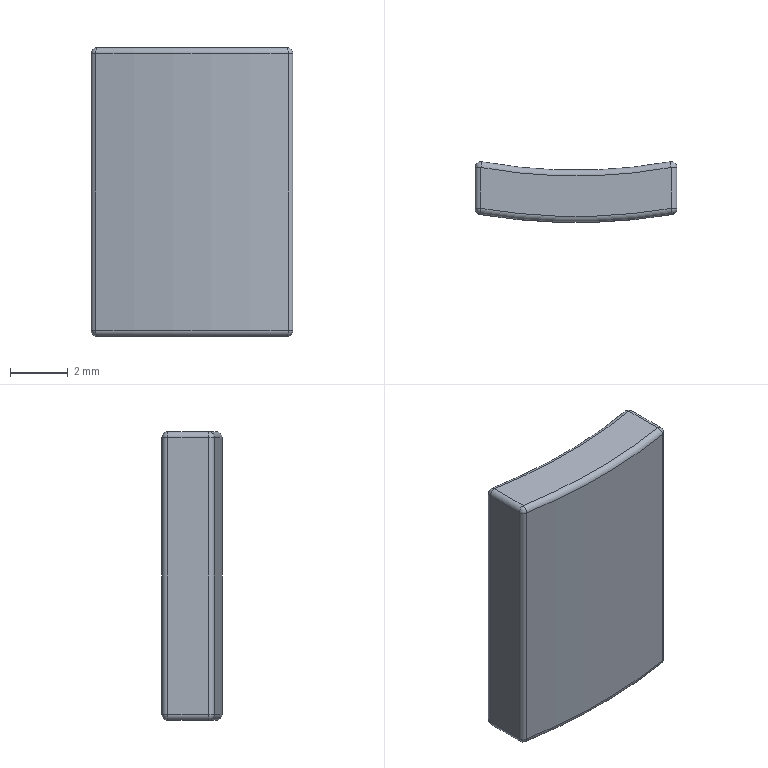Part | SolidWorks | features BaseBody 1 | 1 solid | 26 faces | box 7 x 2.098 x 10 mm | volume 126.049 mm3 | cylinder 10 | sphere 8 | plane 4 | torus 4 | commonest cylinder face diameters 0.4 x8 36.4 x1 40 x1
STEP:
#1=CARTESIAN_POINT('',(-3.3,-18.102,0.));
#2=VERTEX_POINT('',#1);
#3=CARTESIAN_POINT('',(3.3,-18.102,0.));
#4=VERTEX_POINT('',#3);
#5=CARTESIAN_POINT('',(0.,0.,0.));
#6=DIRECTION('',(0.,0.,1.));
#7=DIRECTION('',(-0.1793,-0.9838,0.));
#8=AXIS2_PLACEMENT_3D('',#5,#6,#7);
#9=CIRCLE('',#8,18.4);
#10=EDGE_CURVE('',#2,#4,#9,.T.);
#11=ORIENTED_EDGE('',*,*,#10,.F.);
#12=CARTESIAN_POINT('',(-3.3,-19.523,0.));
#13=VERTEX_POINT('',#12);
#14=CARTESIAN_POINT('',(-3.3,-19.523,0.));
#15=DIRECTION('',(0.,1.,0.));
#16=VECTOR('',#15,1000.);
#17=LINE('',#14,#16);
#18=EDGE_CURVE('',#13,#2,#17,.T.);
#19=ORIENTED_EDGE('',*,*,#18,.F.);
#20=CARTESIAN_POINT('',(3.3,-19.523,0.));
#21=VERTEX_POINT('',#20);
#22=CARTESIAN_POINT('',(0.,0.,0.));
#23=DIRECTION('',(0.,0.,-1.));
#24=DIRECTION('',(0.1667,-0.986,0.));
#25=AXIS2_PLACEMENT_3D('',#22,#23,#24);
#26=CIRCLE('',#25,19.8);
#27=EDGE_CURVE('',#21,#13,#26,.T.);
#28=ORIENTED_EDGE('',*,*,#27,.F.);
#29=CARTESIAN_POINT('',(3.3,-18.102,0.));
#30=DIRECTION('',(0.,-1.,0.));
#31=VECTOR('',#30,1000.);
#32=LINE('',#29,#31);
#33=EDGE_CURVE('',#4,#21,#32,.T.);
#34=ORIENTED_EDGE('',*,*,#33,.F.);
#35=EDGE_LOOP('',(#11,#19,#28,#34));
#36=FACE_OUTER_BOUND('',#35,.T.);
#37=CARTESIAN_POINT('',(0.,0.,0.));
#38=DIRECTION('',(0.,0.,1.));
#39=DIRECTION('',(1.,0.,0.));
#40=AXIS2_PLACEMENT_3D('',#37,#38,#39);
#41=PLANE('',#40);
#42=ADVANCED_FACE('',(#36),#41,.T.);
#43=CARTESIAN_POINT('',(3.3,-18.102,-10.));
#44=VERTEX_POINT('',#43);
#45=CARTESIAN_POINT('',(3.5,-18.102,-9.8));
#46=VERTEX_POINT('',#45);
#47=CARTESIAN_POINT('',(3.3,-18.102,-9.8));
#48=DIRECTION('',(0.,-1.,0.));
#49=DIRECTION('',(0.,0.,-1.));
#50=AXIS2_PLACEMENT_3D('',#47,#48,#49);
#51=CIRCLE('',#50,0.2);
#52=EDGE_CURVE('',#44,#46,#51,.T.);
#53=ORIENTED_EDGE('',*,*,#52,.F.);
#54=CARTESIAN_POINT('',(3.264,-17.905,-9.8));
#55=VERTEX_POINT('',#54);
#56=CARTESIAN_POINT('',(3.3,-18.102,-9.8));
#57=DIRECTION('',(0.9838,0.1793,0.));
#58=DIRECTION('',(0.,0.,-1.));
#59=AXIS2_PLACEMENT_3D('',#56,#57,#58);
#60=CIRCLE('',#59,0.2);
#61=EDGE_CURVE('',#44,#55,#60,.T.);
#62=ORIENTED_EDGE('',*,*,#61,.T.);
#63=CARTESIAN_POINT('',(3.3,-18.102,-9.8));
#64=DIRECTION('',(0.,0.,-1.));
#65=DIRECTION('',(-0.1793,0.9838,0.));
#66=AXIS2_PLACEMENT_3D('',#63,#64,#65);
#67=CIRCLE('',#66,0.2);
#68=EDGE_CURVE('',#55,#46,#67,.T.);
#69=ORIENTED_EDGE('',*,*,#68,.T.);
#70=EDGE_LOOP('',(#53,#62,#69));
#71=FACE_OUTER_BOUND('',#70,.T.);
#72=CARTESIAN_POINT('',(3.3,-18.102,-9.8));
#73=DIRECTION('',(0.,0.,-1.));
#74=DIRECTION('',(0.6406,0.7679,0.));
#75=AXIS2_PLACEMENT_3D('',#72,#73,#74);
#76=SPHERICAL_SURFACE('',#75,0.2);
#77=ADVANCED_FACE('',(#71),#76,.T.);
#78=CARTESIAN_POINT('',(-3.3,-18.102,-10.));
#79=VERTEX_POINT('',#78);
#80=CARTESIAN_POINT('',(-3.264,-17.905,-9.8));
#81=VERTEX_POINT('',#80);
#82=CARTESIAN_POINT('',(-3.3,-18.102,-9.8));
#83=DIRECTION('',(0.9838,-0.1793,0.));
#84=DIRECTION('',(0.,0.,-1.));
#85=AXIS2_PLACEMENT_3D('',#82,#83,#84);
#86=CIRCLE('',#85,0.2);
#87=EDGE_CURVE('',#79,#81,#86,.T.);
#88=ORIENTED_EDGE('',*,*,#87,.T.);
#89=CARTESIAN_POINT('',(0.,0.,-9.8));
#90=DIRECTION('',(0.,0.,1.));
#91=DIRECTION('',(-0.1793,-0.9838,0.));
#92=AXIS2_PLACEMENT_3D('',#89,#90,#91);
#93=CIRCLE('',#92,18.2);
#94=EDGE_CURVE('',#81,#55,#93,.T.);
#95=ORIENTED_EDGE('',*,*,#94,.T.);
#96=ORIENTED_EDGE('',*,*,#61,.F.);
#97=CARTESIAN_POINT('',(0.,0.,-10.));
#98=DIRECTION('',(0.,0.,1.));
#99=DIRECTION('',(-0.1793,-0.9838,0.));
#100=AXIS2_PLACEMENT_3D('',#97,#98,#99);
#101=CIRCLE('',#100,18.4);
#102=EDGE_CURVE('',#79,#44,#101,.T.);
#103=ORIENTED_EDGE('',*,*,#102,.F.);
#104=EDGE_LOOP('',(#88,#95,#96,#103));
#105=FACE_OUTER_BOUND('',#104,.T.);
#106=CARTESIAN_POINT('',(0.,0.,-9.8));
#107=DIRECTION('',(0.,0.,1.));
#108=DIRECTION('',(-0.1841,-0.9829,0.));
#109=AXIS2_PLACEMENT_3D('',#106,#107,#108);
#110=TOROIDAL_SURFACE('',#109,18.4,0.2);
#111=ADVANCED_FACE('',(#105),#110,.T.);
#112=ORIENTED_EDGE('',*,*,#87,.F.);
#113=CARTESIAN_POINT('',(-3.5,-18.102,-9.8));
#114=VERTEX_POINT('',#113);
#115=CARTESIAN_POINT('',(-3.3,-18.102,-9.8));
#116=DIRECTION('',(0.,1.,0.));
#117=DIRECTION('',(0.,0.,-1.));
#118=AXIS2_PLACEMENT_3D('',#115,#116,#117);
#119=CIRCLE('',#118,0.2);
#120=EDGE_CURVE('',#79,#114,#119,.T.);
#121=ORIENTED_EDGE('',*,*,#120,.T.);
#122=CARTESIAN_POINT('',(-3.3,-18.102,-9.8));
#123=DIRECTION('',(0.,0.,-1.));
#124=DIRECTION('',(-1.,0.,0.));
#125=AXIS2_PLACEMENT_3D('',#122,#123,#124);
#126=CIRCLE('',#125,0.2);
#127=EDGE_CURVE('',#114,#81,#126,.T.);
#128=ORIENTED_EDGE('',*,*,#127,.T.);
#129=EDGE_LOOP('',(#112,#121,#128));
#130=FACE_OUTER_BOUND('',#129,.T.);
#131=CARTESIAN_POINT('',(-3.3,-18.102,-9.8));
#132=DIRECTION('',(0.,0.,-1.));
#133=DIRECTION('',(-0.6406,0.7679,0.));
#134=AXIS2_PLACEMENT_3D('',#131,#132,#133);
#135=SPHERICAL_SURFACE('',#134,0.2);
#136=ADVANCED_FACE('',(#130),#135,.T.);
#137=CARTESIAN_POINT('',(-3.3,-19.523,-10.));
#138=VERTEX_POINT('',#137);
#139=CARTESIAN_POINT('',(-3.5,-19.523,-9.8));
#140=VERTEX_POINT('',#139);
#141=CARTESIAN_POINT('',(-3.3,-19.523,-9.8));
#142=DIRECTION('',(0.,1.,0.));
#143=DIRECTION('',(0.,0.,-1.));
#144=AXIS2_PLACEMENT_3D('',#141,#142,#143);
#145=CIRCLE('',#144,0.2);
#146=EDGE_CURVE('',#138,#140,#145,.T.);
#147=ORIENTED_EDGE('',*,*,#146,.T.);
#148=CARTESIAN_POINT('',(-3.5,-19.523,-9.8));
#149=DIRECTION('',(0.,1.,0.));
#150=VECTOR('',#149,1000.);
#151=LINE('',#148,#150);
#152=EDGE_CURVE('',#140,#114,#151,.T.);
#153=ORIENTED_EDGE('',*,*,#152,.T.);
#154=ORIENTED_EDGE('',*,*,#120,.F.);
#155=CARTESIAN_POINT('',(-3.3,-19.523,-10.));
#156=DIRECTION('',(0.,1.,0.));
#157=VECTOR('',#156,1000.);
#158=LINE('',#155,#157);
#159=EDGE_CURVE('',#138,#79,#158,.T.);
#160=ORIENTED_EDGE('',*,*,#159,.F.);
#161=EDGE_LOOP('',(#147,#153,#154,#160));
#162=FACE_OUTER_BOUND('',#161,.T.);
#163=CARTESIAN_POINT('',(-3.3,-19.649,-9.8));
#164=DIRECTION('',(0.,1.,0.));
#165=DIRECTION('',(0.,0.,-1.));
#166=AXIS2_PLACEMENT_3D('',#163,#164,#165);
#167=CYLINDRICAL_SURFACE('',#166,0.2);
#168=ADVANCED_FACE('',(#162),#167,.T.);
#169=CARTESIAN_POINT('',(-3.5,-18.102,-0.2));
#170=VERTEX_POINT('',#169);
#171=CARTESIAN_POINT('',(-3.5,-18.102,-9.8));
#172=DIRECTION('',(0.,0.,1.));
#173=VECTOR('',#172,1000.);
#174=LINE('',#171,#173);
#175=EDGE_CURVE('',#114,#170,#174,.T.);
#176=ORIENTED_EDGE('',*,*,#175,.F.);
#177=ORIENTED_EDGE('',*,*,#152,.F.);
#178=CARTESIAN_POINT('',(-3.5,-19.523,-0.2));
#179=VERTEX_POINT('',#178);
#180=CARTESIAN_POINT('',(-3.5,-19.523,-0.2));
#181=DIRECTION('',(0.,0.,-1.));
#182=VECTOR('',#181,1000.);
#183=LINE('',#180,#182);
#184=EDGE_CURVE('',#179,#140,#183,.T.);
#185=ORIENTED_EDGE('',*,*,#184,.F.);
#186=CARTESIAN_POINT('',(-3.5,-19.523,-0.2));
#187=DIRECTION('',(0.,1.,0.));
#188=VECTOR('',#187,1000.);
#189=LINE('',#186,#188);
#190=EDGE_CURVE('',#179,#170,#189,.T.);
#191=ORIENTED_EDGE('',*,*,#190,.T.);
#192=EDGE_LOOP('',(#176,#177,#185,#191));
#193=FACE_OUTER_BOUND('',#192,.T.);
#194=CARTESIAN_POINT('',(-3.5,-15.854,-10.));
#195=DIRECTION('',(1.,0.,0.));
#196=DIRECTION('',(0.,1.,0.));
#197=AXIS2_PLACEMENT_3D('',#194,#195,#196);
#198=PLANE('',#197);
#199=ADVANCED_FACE('',(#193),#198,.F.);
#200=CARTESIAN_POINT('',(-3.3,-19.523,-0.2));
#201=DIRECTION('',(0.,1.,0.));
#202=DIRECTION('',(-1.,0.,0.));
#203=AXIS2_PLACEMENT_3D('',#200,#201,#202);
#204=CIRCLE('',#203,0.2);
#205=EDGE_CURVE('',#179,#13,#204,.T.);
#206=ORIENTED_EDGE('',*,*,#205,.T.);
#207=ORIENTED_EDGE('',*,*,#18,.T.);
#208=CARTESIAN_POINT('',(-3.3,-18.102,-0.2));
#209=DIRECTION('',(0.,1.,0.));
#210=DIRECTION('',(-1.,0.,0.));
#211=AXIS2_PLACEMENT_3D('',#208,#209,#210);
#212=CIRCLE('',#211,0.2);
#213=EDGE_CURVE('',#170,#2,#212,.T.);
#214=ORIENTED_EDGE('',*,*,#213,.F.);
#215=ORIENTED_EDGE('',*,*,#190,.F.);
#216=EDGE_LOOP('',(#206,#207,#214,#215));
#217=FACE_OUTER_BOUND('',#216,.T.);
#218=CARTESIAN_POINT('',(-3.3,-19.608,-0.2));
#219=DIRECTION('',(0.,1.,0.));
#220=DIRECTION('',(-1.,0.,0.));
#221=AXIS2_PLACEMENT_3D('',#218,#219,#220);
#222=CYLINDRICAL_SURFACE('',#221,0.2);
#223=ADVANCED_FACE('',(#217),#222,.T.);
#224=ORIENTED_EDGE('',*,*,#213,.T.);
#225=CARTESIAN_POINT('',(-3.264,-17.905,-0.2));
#226=VERTEX_POINT('',#225);
#227=CARTESIAN_POINT('',(-3.3,-18.102,-0.2));
#228=DIRECTION('',(0.9838,-0.1793,0.));
#229=DIRECTION('',(0.1793,0.9838,0.));
#230=AXIS2_PLACEMENT_3D('',#227,#228,#229);
#231=CIRCLE('',#230,0.2);
#232=EDGE_CURVE('',#226,#2,#231,.T.);
#233=ORIENTED_EDGE('',*,*,#232,.F.);
#234=CARTESIAN_POINT('',(-3.3,-18.102,-0.2));
#235=DIRECTION('',(0.,0.,-1.));
#236=DIRECTION('',(-1.,0.,0.));
#237=AXIS2_PLACEMENT_3D('',#234,#235,#236);
#238=CIRCLE('',#237,0.2);
#239=EDGE_CURVE('',#170,#226,#238,.T.);
#240=ORIENTED_EDGE('',*,*,#239,.F.);
#241=EDGE_LOOP('',(#224,#233,#240));
#242=FACE_OUTER_BOUND('',#241,.T.);
#243=CARTESIAN_POINT('',(-3.3,-18.102,-0.2));
#244=DIRECTION('',(0.,0.,-1.));
#245=DIRECTION('',(-0.6406,0.7679,0.));
#246=AXIS2_PLACEMENT_3D('',#243,#244,#245);
#247=SPHERICAL_SURFACE('',#246,0.2);
#248=ADVANCED_FACE('',(#242),#247,.T.);
#249=CARTESIAN_POINT('',(-3.264,-17.905,-9.8));
#250=DIRECTION('',(0.,0.,1.));
#251=VECTOR('',#250,1000.);
#252=LINE('',#249,#251);
#253=EDGE_CURVE('',#81,#226,#252,.T.);
#254=ORIENTED_EDGE('',*,*,#253,.F.);
#255=ORIENTED_EDGE('',*,*,#127,.F.);
#256=ORIENTED_EDGE('',*,*,#175,.T.);
#257=ORIENTED_EDGE('',*,*,#239,.T.);
#258=EDGE_LOOP('',(#254,#255,#256,#257));
#259=FACE_OUTER_BOUND('',#258,.T.);
#260=CARTESIAN_POINT('',(-3.3,-18.102,-23.036));
#261=DIRECTION('',(0.,0.,1.));
#262=DIRECTION('',(0.1793,0.9838,0.));
#263=AXIS2_PLACEMENT_3D('',#260,#261,#262);
#264=CYLINDRICAL_SURFACE('',#263,0.2);
#265=ADVANCED_FACE('',(#259),#264,.T.);
#266=CARTESIAN_POINT('',(3.264,-17.905,-0.2));
#267=VERTEX_POINT('',#266);
#268=CARTESIAN_POINT('',(3.264,-17.905,-0.2));
#269=DIRECTION('',(0.,0.,-1.));
#270=VECTOR('',#269,1000.);
#271=LINE('',#268,#270);
#272=EDGE_CURVE('',#267,#55,#271,.T.);
#273=ORIENTED_EDGE('',*,*,#272,.T.);
#274=ORIENTED_EDGE('',*,*,#94,.F.);
#275=ORIENTED_EDGE('',*,*,#253,.T.);
#276=CARTESIAN_POINT('',(0.,0.,-0.2));
#277=DIRECTION('',(0.,0.,1.));
#278=DIRECTION('',(-0.1793,-0.9838,0.));
#279=AXIS2_PLACEMENT_3D('',#276,#277,#278);
#280=CIRCLE('',#279,18.2);
#281=EDGE_CURVE('',#226,#267,#280,.T.);
#282=ORIENTED_EDGE('',*,*,#281,.T.);
#283=EDGE_LOOP('',(#273,#274,#275,#282));
#284=FACE_OUTER_BOUND('',#283,.T.);
#285=CARTESIAN_POINT('',(0.,0.,-10.5));
#286=DIRECTION('',(0.,0.,1.));
#287=DIRECTION('',(-1.,0.,0.));
#288=AXIS2_PLACEMENT_3D('',#285,#286,#287);
#289=CYLINDRICAL_SURFACE('',#288,18.2);
#290=ADVANCED_FACE('',(#284),#289,.F.);
#291=ORIENTED_EDGE('',*,*,#232,.T.);
#292=ORIENTED_EDGE('',*,*,#10,.T.);
#293=CARTESIAN_POINT('',(3.3,-18.102,-0.2));
#294=DIRECTION('',(0.9838,0.1793,0.));
#295=DIRECTION('',(-0.1793,0.9838,0.));
#296=AXIS2_PLACEMENT_3D('',#293,#294,#295);
#297=CIRCLE('',#296,0.2);
#298=EDGE_CURVE('',#267,#4,#297,.T.);
#299=ORIENTED_EDGE('',*,*,#298,.F.);
#300=ORIENTED_EDGE('',*,*,#281,.F.);
#301=EDGE_LOOP('',(#291,#292,#299,#300));
#302=FACE_OUTER_BOUND('',#301,.T.);
#303=CARTESIAN_POINT('',(0.,0.,-0.2));
#304=DIRECTION('',(0.,0.,1.));
#305=DIRECTION('',(-0.1844,-0.9829,0.));
#306=AXIS2_PLACEMENT_3D('',#303,#304,#305);
#307=TOROIDAL_SURFACE('',#306,18.4,0.2);
#308=ADVANCED_FACE('',(#302),#307,.T.);
#309=ORIENTED_EDGE('',*,*,#298,.T.);
#310=CARTESIAN_POINT('',(3.5,-18.102,-0.2));
#311=VERTEX_POINT('',#310);
#312=CARTESIAN_POINT('',(3.3,-18.102,-0.2));
#313=DIRECTION('',(0.,-1.,0.));
#314=DIRECTION('',(1.,0.,0.));
#315=AXIS2_PLACEMENT_3D('',#312,#313,#314);
#316=CIRCLE('',#315,0.2);
#317=EDGE_CURVE('',#311,#4,#316,.T.);
#318=ORIENTED_EDGE('',*,*,#317,.F.);
#319=CARTESIAN_POINT('',(3.3,-18.102,-0.2));
#320=DIRECTION('',(0.,0.,-1.));
#321=DIRECTION('',(-0.1793,0.9838,0.));
#322=AXIS2_PLACEMENT_3D('',#319,#320,#321);
#323=CIRCLE('',#322,0.2);
#324=EDGE_CURVE('',#267,#311,#323,.T.);
#325=ORIENTED_EDGE('',*,*,#324,.F.);
#326=EDGE_LOOP('',(#309,#318,#325));
#327=FACE_OUTER_BOUND('',#326,.T.);
#328=CARTESIAN_POINT('',(3.3,-18.102,-0.2));
#329=DIRECTION('',(0.,0.,-1.));
#330=DIRECTION('',(0.6406,0.7679,0.));
#331=AXIS2_PLACEMENT_3D('',#328,#329,#330);
#332=SPHERICAL_SURFACE('',#331,0.2);
#333=ADVANCED_FACE('',(#327),#332,.T.);
#334=CARTESIAN_POINT('',(3.5,-18.102,-0.2));
#335=DIRECTION('',(0.,0.,-1.));
#336=VECTOR('',#335,1000.);
#337=LINE('',#334,#336);
#338=EDGE_CURVE('',#311,#46,#337,.T.);
#339=ORIENTED_EDGE('',*,*,#338,.T.);
#340=ORIENTED_EDGE('',*,*,#68,.F.);
#341=ORIENTED_EDGE('',*,*,#272,.F.);
#342=ORIENTED_EDGE('',*,*,#324,.T.);
#343=EDGE_LOOP('',(#339,#340,#341,#342));
#344=FACE_OUTER_BOUND('',#343,.T.);
#345=CARTESIAN_POINT('',(3.3,-18.102,13.036));
#346=DIRECTION('',(0.,0.,-1.));
#347=DIRECTION('',(-0.1793,0.9838,0.));
#348=AXIS2_PLACEMENT_3D('',#345,#346,#347);
#349=CYLINDRICAL_SURFACE('',#348,0.2);
#350=ADVANCED_FACE('',(#344),#349,.T.);
#351=CARTESIAN_POINT('',(3.5,-19.523,-9.8));
#352=VERTEX_POINT('',#351);
#353=CARTESIAN_POINT('',(3.5,-19.523,-0.2));
#354=VERTEX_POINT('',#353);
#355=CARTESIAN_POINT('',(3.5,-19.523,-9.8));
#356=DIRECTION('',(0.,0.,1.));
#357=VECTOR('',#356,1000.);
#358=LINE('',#355,#357);
#359=EDGE_CURVE('',#352,#354,#358,.T.);
#360=ORIENTED_EDGE('',*,*,#359,.F.);
#361=CARTESIAN_POINT('',(3.5,-18.102,-9.8));
#362=DIRECTION('',(0.,-1.,0.));
#363=VECTOR('',#362,1000.);
#364=LINE('',#361,#363);
#365=EDGE_CURVE('',#46,#352,#364,.T.);
#366=ORIENTED_EDGE('',*,*,#365,.F.);
#367=ORIENTED_EDGE('',*,*,#338,.F.);
#368=CARTESIAN_POINT('',(3.5,-18.102,-0.2));
#369=DIRECTION('',(0.,-1.,0.));
#370=VECTOR('',#369,1000.);
#371=LINE('',#368,#370);
#372=EDGE_CURVE('',#311,#354,#371,.T.);
#373=ORIENTED_EDGE('',*,*,#372,.T.);
#374=EDGE_LOOP('',(#360,#366,#367,#373));
#375=FACE_OUTER_BOUND('',#374,.T.);
#376=CARTESIAN_POINT('',(3.5,-22.259,-10.));
#377=DIRECTION('',(-1.,0.,0.));
#378=DIRECTION('',(0.,0.,1.));
#379=AXIS2_PLACEMENT_3D('',#376,#377,#378);
#380=PLANE('',#379);
#381=ADVANCED_FACE('',(#375),#380,.F.);
#382=ORIENTED_EDGE('',*,*,#317,.T.);
#383=ORIENTED_EDGE('',*,*,#33,.T.);
#384=CARTESIAN_POINT('',(3.3,-19.523,-0.2));
#385=DIRECTION('',(0.,-1.,0.));
#386=DIRECTION('',(1.,0.,0.));
#387=AXIS2_PLACEMENT_3D('',#384,#385,#386);
#388=CIRCLE('',#387,0.2);
#389=EDGE_CURVE('',#354,#21,#388,.T.);
#390=ORIENTED_EDGE('',*,*,#389,.F.);
#391=ORIENTED_EDGE('',*,*,#372,.F.);
#392=EDGE_LOOP('',(#382,#383,#390,#391));
#393=FACE_OUTER_BOUND('',#392,.T.);
#394=CARTESIAN_POINT('',(3.3,-18.017,-0.2));
#395=DIRECTION('',(0.,-1.,0.));
#396=DIRECTION('',(1.,0.,0.));
#397=AXIS2_PLACEMENT_3D('',#394,#395,#396);
#398=CYLINDRICAL_SURFACE('',#397,0.2);
#399=ADVANCED_FACE('',(#393),#398,.T.);
#400=ORIENTED_EDGE('',*,*,#389,.T.);
#401=CARTESIAN_POINT('',(3.333,-19.72,-0.2));
#402=VERTEX_POINT('',#401);
#403=CARTESIAN_POINT('',(3.3,-19.523,-0.2));
#404=DIRECTION('',(-0.986,-0.1667,0.));
#405=DIRECTION('',(0.1667,-0.986,0.));
#406=AXIS2_PLACEMENT_3D('',#403,#404,#405);
#407=CIRCLE('',#406,0.2);
#408=EDGE_CURVE('',#402,#21,#407,.T.);
#409=ORIENTED_EDGE('',*,*,#408,.F.);
#410=CARTESIAN_POINT('',(3.3,-19.523,-0.2));
#411=DIRECTION('',(0.,0.,-1.));
#412=DIRECTION('',(1.,0.,0.));
#413=AXIS2_PLACEMENT_3D('',#410,#411,#412);
#414=CIRCLE('',#413,0.2);
#415=EDGE_CURVE('',#354,#402,#414,.T.);
#416=ORIENTED_EDGE('',*,*,#415,.F.);
#417=EDGE_LOOP('',(#400,#409,#416));
#418=FACE_OUTER_BOUND('',#417,.T.);
#419=CARTESIAN_POINT('',(3.3,-19.523,-0.2));
#420=DIRECTION('',(0.,0.,-1.));
#421=DIRECTION('',(0.7638,-0.6455,0.));
#422=AXIS2_PLACEMENT_3D('',#419,#420,#421);
#423=SPHERICAL_SURFACE('',#422,0.2);
#424=ADVANCED_FACE('',(#418),#423,.T.);
#425=CARTESIAN_POINT('',(3.333,-19.72,-9.8));
#426=VERTEX_POINT('',#425);
#427=CARTESIAN_POINT('',(3.333,-19.72,-9.8));
#428=DIRECTION('',(0.,0.,1.));
#429=VECTOR('',#428,1000.);
#430=LINE('',#427,#429);
#431=EDGE_CURVE('',#426,#402,#430,.T.);
#432=ORIENTED_EDGE('',*,*,#431,.F.);
#433=CARTESIAN_POINT('',(3.3,-19.523,-9.8));
#434=DIRECTION('',(0.,0.,-1.));
#435=DIRECTION('',(1.,0.,0.));
#436=AXIS2_PLACEMENT_3D('',#433,#434,#435);
#437=CIRCLE('',#436,0.2);
#438=EDGE_CURVE('',#352,#426,#437,.T.);
#439=ORIENTED_EDGE('',*,*,#438,.F.);
#440=ORIENTED_EDGE('',*,*,#359,.T.);
#441=ORIENTED_EDGE('',*,*,#415,.T.);
#442=EDGE_LOOP('',(#432,#439,#440,#441));
#443=FACE_OUTER_BOUND('',#442,.T.);
#444=CARTESIAN_POINT('',(3.3,-19.523,-23.036));
#445=DIRECTION('',(0.,0.,1.));
#446=DIRECTION('',(0.1667,-0.986,0.));
#447=AXIS2_PLACEMENT_3D('',#444,#445,#446);
#448=CYLINDRICAL_SURFACE('',#447,0.2);
#449=ADVANCED_FACE('',(#443),#448,.T.);
#450=CARTESIAN_POINT('',(3.3,-19.523,-10.));
#451=VERTEX_POINT('',#450);
#452=CARTESIAN_POINT('',(3.3,-19.523,-9.8));
#453=DIRECTION('',(-0.986,-0.1667,0.));
#454=DIRECTION('',(0.,0.,-1.));
#455=AXIS2_PLACEMENT_3D('',#452,#453,#454);
#456=CIRCLE('',#455,0.2);
#457=EDGE_CURVE('',#451,#426,#456,.T.);
#458=ORIENTED_EDGE('',*,*,#457,.F.);
#459=CARTESIAN_POINT('',(3.3,-19.523,-9.8));
#460=DIRECTION('',(0.,-1.,0.));
#461=DIRECTION('',(0.,0.,-1.));
#462=AXIS2_PLACEMENT_3D('',#459,#460,#461);
#463=CIRCLE('',#462,0.2);
#464=EDGE_CURVE('',#451,#352,#463,.T.);
#465=ORIENTED_EDGE('',*,*,#464,.T.);
#466=ORIENTED_EDGE('',*,*,#438,.T.);
#467=EDGE_LOOP('',(#458,#465,#466));
#468=FACE_OUTER_BOUND('',#467,.T.);
#469=CARTESIAN_POINT('',(3.3,-19.523,-9.8));
#470=DIRECTION('',(0.,0.,-1.));
#471=DIRECTION('',(0.7638,-0.6455,0.));
#472=AXIS2_PLACEMENT_3D('',#469,#470,#471);
#473=SPHERICAL_SURFACE('',#472,0.2);
#474=ADVANCED_FACE('',(#468),#473,.T.);
#475=ORIENTED_EDGE('',*,*,#52,.T.);
#476=ORIENTED_EDGE('',*,*,#365,.T.);
#477=ORIENTED_EDGE('',*,*,#464,.F.);
#478=CARTESIAN_POINT('',(3.3,-18.102,-10.));
#479=DIRECTION('',(0.,-1.,0.));
#480=VECTOR('',#479,1000.);
#481=LINE('',#478,#480);
#482=EDGE_CURVE('',#44,#451,#481,.T.);
#483=ORIENTED_EDGE('',*,*,#482,.F.);
#484=EDGE_LOOP('',(#475,#476,#477,#483));
#485=FACE_OUTER_BOUND('',#484,.T.);
#486=CARTESIAN_POINT('',(3.3,-17.976,-9.8));
#487=DIRECTION('',(0.,-1.,0.));
#488=DIRECTION('',(0.,0.,-1.));
#489=AXIS2_PLACEMENT_3D('',#486,#487,#488);
#490=CYLINDRICAL_SURFACE('',#489,0.2);
#491=ADVANCED_FACE('',(#485),#490,.T.);
#492=CARTESIAN_POINT('',(0.,0.,-10.));
#493=DIRECTION('',(0.,0.,-1.));
#494=DIRECTION('',(0.1667,-0.986,0.));
#495=AXIS2_PLACEMENT_3D('',#492,#493,#494);
#496=CIRCLE('',#495,19.8);
#497=EDGE_CURVE('',#451,#138,#496,.T.);
#498=ORIENTED_EDGE('',*,*,#497,.T.);
#499=ORIENTED_EDGE('',*,*,#159,.T.);
#500=ORIENTED_EDGE('',*,*,#102,.T.);
#501=ORIENTED_EDGE('',*,*,#482,.T.);
#502=EDGE_LOOP('',(#498,#499,#500,#501));
#503=FACE_OUTER_BOUND('',#502,.T.);
#504=CARTESIAN_POINT('',(0.,0.,-10.));
#505=DIRECTION('',(0.,0.,1.));
#506=DIRECTION('',(1.,0.,0.));
#507=AXIS2_PLACEMENT_3D('',#504,#505,#506);
#508=PLANE('',#507);
#509=ADVANCED_FACE('',(#503),#508,.F.);
#510=ORIENTED_EDGE('',*,*,#457,.T.);
#511=CARTESIAN_POINT('',(-3.333,-19.72,-9.8));
#512=VERTEX_POINT('',#511);
#513=CARTESIAN_POINT('',(0.,0.,-9.8));
#514=DIRECTION('',(0.,0.,-1.));
#515=DIRECTION('',(0.1667,-0.986,0.));
#516=AXIS2_PLACEMENT_3D('',#513,#514,#515);
#517=CIRCLE('',#516,20.);
#518=EDGE_CURVE('',#426,#512,#517,.T.);
#519=ORIENTED_EDGE('',*,*,#518,.T.);
#520=CARTESIAN_POINT('',(-3.3,-19.523,-9.8));
#521=DIRECTION('',(-0.986,0.1667,0.));
#522=DIRECTION('',(0.,0.,-1.));
#523=AXIS2_PLACEMENT_3D('',#520,#521,#522);
#524=CIRCLE('',#523,0.2);
#525=EDGE_CURVE('',#138,#512,#524,.T.);
#526=ORIENTED_EDGE('',*,*,#525,.F.);
#527=ORIENTED_EDGE('',*,*,#497,.F.);
#528=EDGE_LOOP('',(#510,#519,#526,#527));
#529=FACE_OUTER_BOUND('',#528,.T.);
#530=CARTESIAN_POINT('',(0.,0.,-9.8));
#531=DIRECTION('',(0.,0.,1.));
#532=DIRECTION('',(0.1729,-0.9849,0.));
#533=AXIS2_PLACEMENT_3D('',#530,#531,#532);
#534=TOROIDAL_SURFACE('',#533,19.8,0.2);
#535=ADVANCED_FACE('',(#529),#534,.T.);
#536=ORIENTED_EDGE('',*,*,#146,.F.);
#537=ORIENTED_EDGE('',*,*,#525,.T.);
#538=CARTESIAN_POINT('',(-3.3,-19.523,-9.8));
#539=DIRECTION('',(0.,0.,-1.));
#540=DIRECTION('',(-0.1667,-0.986,0.));
#541=AXIS2_PLACEMENT_3D('',#538,#539,#540);
#542=CIRCLE('',#541,0.2);
#543=EDGE_CURVE('',#512,#140,#542,.T.);
#544=ORIENTED_EDGE('',*,*,#543,.T.);
#545=EDGE_LOOP('',(#536,#537,#544));
#546=FACE_OUTER_BOUND('',#545,.T.);
#547=CARTESIAN_POINT('',(-3.3,-19.523,-9.8));
#548=DIRECTION('',(0.,0.,-1.));
#549=DIRECTION('',(-0.7638,-0.6455,0.));
#550=AXIS2_PLACEMENT_3D('',#547,#548,#549);
#551=SPHERICAL_SURFACE('',#550,0.2);
#552=ADVANCED_FACE('',(#546),#551,.T.);
#553=ORIENTED_EDGE('',*,*,#184,.T.);
#554=ORIENTED_EDGE('',*,*,#543,.F.);
#555=CARTESIAN_POINT('',(-3.333,-19.72,-0.2));
#556=VERTEX_POINT('',#555);
#557=CARTESIAN_POINT('',(-3.333,-19.72,-0.2));
#558=DIRECTION('',(0.,0.,-1.));
#559=VECTOR('',#558,1000.);
#560=LINE('',#557,#559);
#561=EDGE_CURVE('',#556,#512,#560,.T.);
#562=ORIENTED_EDGE('',*,*,#561,.F.);
#563=CARTESIAN_POINT('',(-3.3,-19.523,-0.2));
#564=DIRECTION('',(0.,0.,-1.));
#565=DIRECTION('',(-0.1667,-0.986,0.));
#566=AXIS2_PLACEMENT_3D('',#563,#564,#565);
#567=CIRCLE('',#566,0.2);
#568=EDGE_CURVE('',#556,#179,#567,.T.);
#569=ORIENTED_EDGE('',*,*,#568,.T.);
#570=EDGE_LOOP('',(#553,#554,#562,#569));
#571=FACE_OUTER_BOUND('',#570,.T.);
#572=CARTESIAN_POINT('',(-3.3,-19.523,13.036));
#573=DIRECTION('',(0.,0.,-1.));
#574=DIRECTION('',(-0.1667,-0.986,0.));
#575=AXIS2_PLACEMENT_3D('',#572,#573,#574);
#576=CYLINDRICAL_SURFACE('',#575,0.2);
#577=ADVANCED_FACE('',(#571),#576,.T.);
#578=CARTESIAN_POINT('',(-3.3,-19.523,-0.2));
#579=DIRECTION('',(-0.986,0.1667,0.));
#580=DIRECTION('',(-0.1667,-0.986,0.));
#581=AXIS2_PLACEMENT_3D('',#578,#579,#580);
#582=CIRCLE('',#581,0.2);
#583=EDGE_CURVE('',#556,#13,#582,.T.);
#584=ORIENTED_EDGE('',*,*,#583,.T.);
#585=ORIENTED_EDGE('',*,*,#205,.F.);
#586=ORIENTED_EDGE('',*,*,#568,.F.);
#587=EDGE_LOOP('',(#584,#585,#586));
#588=FACE_OUTER_BOUND('',#587,.T.);
#589=CARTESIAN_POINT('',(-3.3,-19.523,-0.2));
#590=DIRECTION('',(0.,0.,-1.));
#591=DIRECTION('',(-0.7638,-0.6455,0.));
#592=AXIS2_PLACEMENT_3D('',#589,#590,#591);
#593=SPHERICAL_SURFACE('',#592,0.2);
#594=ADVANCED_FACE('',(#588),#593,.T.);
#595=ORIENTED_EDGE('',*,*,#408,.T.);
#596=ORIENTED_EDGE('',*,*,#27,.T.);
#597=ORIENTED_EDGE('',*,*,#583,.F.);
#598=CARTESIAN_POINT('',(0.,0.,-0.2));
#599=DIRECTION('',(0.,0.,-1.));
#600=DIRECTION('',(0.1667,-0.986,0.));
#601=AXIS2_PLACEMENT_3D('',#598,#599,#600);
#602=CIRCLE('',#601,20.);
#603=EDGE_CURVE('',#402,#556,#602,.T.);
#604=ORIENTED_EDGE('',*,*,#603,.F.);
#605=EDGE_LOOP('',(#595,#596,#597,#604));
#606=FACE_OUTER_BOUND('',#605,.T.);
#607=CARTESIAN_POINT('',(0.,0.,-0.2));
#608=DIRECTION('',(0.,0.,1.));
#609=DIRECTION('',(0.1709,-0.9853,0.));
#610=AXIS2_PLACEMENT_3D('',#607,#608,#609);
#611=TOROIDAL_SURFACE('',#610,19.8,0.2);
#612=ADVANCED_FACE('',(#606),#611,.T.);
#613=ORIENTED_EDGE('',*,*,#561,.T.);
#614=ORIENTED_EDGE('',*,*,#518,.F.);
#615=ORIENTED_EDGE('',*,*,#431,.T.);
#616=ORIENTED_EDGE('',*,*,#603,.T.);
#617=EDGE_LOOP('',(#613,#614,#615,#616));
#618=FACE_OUTER_BOUND('',#617,.T.);
#619=CARTESIAN_POINT('',(0.,0.,-10.5));
#620=DIRECTION('',(0.,0.,1.));
#621=DIRECTION('',(-1.,0.,0.));
#622=AXIS2_PLACEMENT_3D('',#619,#620,#621);
#623=CYLINDRICAL_SURFACE('',#622,20.);
#624=ADVANCED_FACE('',(#618),#623,.T.);
#625=CLOSED_SHELL('',(#42,#77,#111,#136,#168,#199,#223,#248,#265,#290,#308,#333,#350,#381,#399,#424,#449,#474,#491,#509,#535,#552,#577,#594,#612,#624));
#626=MANIFOLD_SOLID_BREP('',#625);
#627=CARTESIAN_POINT('',(0.,0.,0.));
#628=DIRECTION('',(0.,0.,1.));
#629=DIRECTION('',(1.,0.,0.));
#630=AXIS2_PLACEMENT_3D('',#627,#628,#629);
#631=(LENGTH_UNIT()NAMED_UNIT(*)SI_UNIT(.MILLI.,.METRE.));
#632=UNCERTAINTY_MEASURE_WITH_UNIT(LENGTH_MEASURE(0.00001),#631,'','');
#633=(NAMED_UNIT(*)PLANE_ANGLE_UNIT()SI_UNIT($,.RADIAN.));
#634=(NAMED_UNIT(*)SI_UNIT($,.STERADIAN.)SOLID_ANGLE_UNIT());
#635=(GEOMETRIC_REPRESENTATION_CONTEXT(3)GLOBAL_UNCERTAINTY_ASSIGNED_CONTEXT((#632))GLOBAL_UNIT_ASSIGNED_CONTEXT((#631,#633,#634))REPRESENTATION_CONTEXT('',''));
#636=ADVANCED_BREP_SHAPE_REPRESENTATION('',(#626,#630),#635);